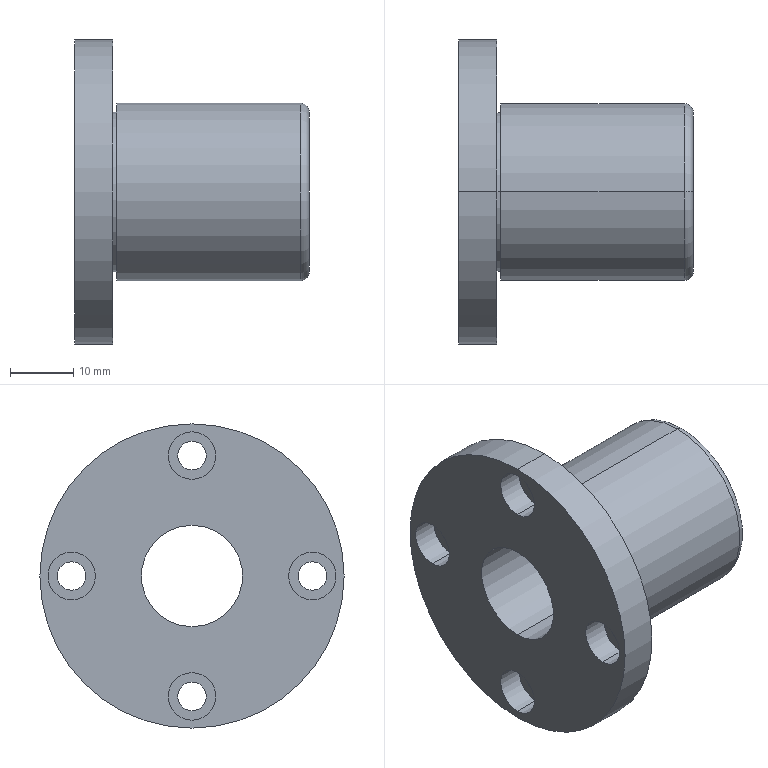Part | STEP file | MFMS16 | 1 solid | 34 faces | box 37 x 48 x 48 mm | volume 21555 mm3 | cylinder 24 | plane 8 | torus 2 | commonest cylinder face diameters 4.5 x8 7.5 x8 16 x2 25.2 x2 28 x2 48 x2
STEP:
#1=CARTESIAN_POINT('',(6.,0.,16.75));
#2=VERTEX_POINT('',#1);
#3=CARTESIAN_POINT('',(6.,0.,21.25));
#4=VERTEX_POINT('',#3);
#5=CARTESIAN_POINT('',(6.,0.,19.));
#6=DIRECTION('',(-1.,0.,0.));
#7=DIRECTION('',(0.,0.,1.));
#8=AXIS2_PLACEMENT_3D('',#5,#6,#7);
#9=CIRCLE('',#8,2.25);
#10=EDGE_CURVE('',#2,#4,#9,.T.);
#11=ORIENTED_EDGE('',*,*,#10,.F.);
#12=CARTESIAN_POINT('',(4.1,0.,16.75));
#13=VERTEX_POINT('',#12);
#14=CARTESIAN_POINT('',(6.,0.,16.75));
#15=DIRECTION('',(-1.,0.,0.));
#16=VECTOR('',#15,1000.);
#17=LINE('',#14,#16);
#18=EDGE_CURVE('',#2,#13,#17,.T.);
#19=ORIENTED_EDGE('',*,*,#18,.T.);
#20=CARTESIAN_POINT('',(4.1,0.,21.25));
#21=VERTEX_POINT('',#20);
#22=CARTESIAN_POINT('',(4.1,0.,19.));
#23=DIRECTION('',(-1.,0.,0.));
#24=DIRECTION('',(0.,0.,1.));
#25=AXIS2_PLACEMENT_3D('',#22,#23,#24);
#26=CIRCLE('',#25,2.25);
#27=EDGE_CURVE('',#13,#21,#26,.T.);
#28=ORIENTED_EDGE('',*,*,#27,.T.);
#29=CARTESIAN_POINT('',(6.,0.,21.25));
#30=DIRECTION('',(-1.,0.,0.));
#31=VECTOR('',#30,1000.);
#32=LINE('',#29,#31);
#33=EDGE_CURVE('',#4,#21,#32,.T.);
#34=ORIENTED_EDGE('',*,*,#33,.F.);
#35=EDGE_LOOP('',(#11,#19,#28,#34));
#36=FACE_OUTER_BOUND('',#35,.T.);
#37=CARTESIAN_POINT('',(6.,0.,19.));
#38=DIRECTION('',(-1.,0.,0.));
#39=DIRECTION('',(0.,0.,1.));
#40=AXIS2_PLACEMENT_3D('',#37,#38,#39);
#41=CYLINDRICAL_SURFACE('',#40,2.25);
#42=ADVANCED_FACE('',(#36),#41,.F.);
#43=CARTESIAN_POINT('',(4.1,0.,15.25));
#44=VERTEX_POINT('',#43);
#45=CARTESIAN_POINT('',(4.1,0.,22.75));
#46=VERTEX_POINT('',#45);
#47=CARTESIAN_POINT('',(4.1,0.,19.));
#48=DIRECTION('',(-1.,0.,0.));
#49=DIRECTION('',(0.,0.,1.));
#50=AXIS2_PLACEMENT_3D('',#47,#48,#49);
#51=CIRCLE('',#50,3.75);
#52=EDGE_CURVE('',#44,#46,#51,.T.);
#53=ORIENTED_EDGE('',*,*,#52,.F.);
#54=CARTESIAN_POINT('',(0.,0.,15.25));
#55=VERTEX_POINT('',#54);
#56=CARTESIAN_POINT('',(6.,0.,15.25));
#57=DIRECTION('',(-1.,0.,0.));
#58=VECTOR('',#57,1000.);
#59=LINE('',#56,#58);
#60=EDGE_CURVE('',#44,#55,#59,.T.);
#61=ORIENTED_EDGE('',*,*,#60,.T.);
#62=CARTESIAN_POINT('',(0.,0.,22.75));
#63=VERTEX_POINT('',#62);
#64=CARTESIAN_POINT('',(0.,0.,19.));
#65=DIRECTION('',(-1.,0.,0.));
#66=DIRECTION('',(0.,0.,1.));
#67=AXIS2_PLACEMENT_3D('',#64,#65,#66);
#68=CIRCLE('',#67,3.75);
#69=EDGE_CURVE('',#55,#63,#68,.T.);
#70=ORIENTED_EDGE('',*,*,#69,.T.);
#71=CARTESIAN_POINT('',(6.,0.,22.75));
#72=DIRECTION('',(-1.,0.,0.));
#73=VECTOR('',#72,1000.);
#74=LINE('',#71,#73);
#75=EDGE_CURVE('',#46,#63,#74,.T.);
#76=ORIENTED_EDGE('',*,*,#75,.F.);
#77=EDGE_LOOP('',(#53,#61,#70,#76));
#78=FACE_OUTER_BOUND('',#77,.T.);
#79=CARTESIAN_POINT('',(6.,0.,19.));
#80=DIRECTION('',(-1.,0.,0.));
#81=DIRECTION('',(0.,0.,1.));
#82=AXIS2_PLACEMENT_3D('',#79,#80,#81);
#83=CYLINDRICAL_SURFACE('',#82,3.75);
#84=ADVANCED_FACE('',(#78),#83,.F.);
#85=CARTESIAN_POINT('',(6.,-19.,-2.25));
#86=VERTEX_POINT('',#85);
#87=CARTESIAN_POINT('',(6.,-19.,2.25));
#88=VERTEX_POINT('',#87);
#89=CARTESIAN_POINT('',(6.,-19.,0.));
#90=DIRECTION('',(-1.,0.,0.));
#91=DIRECTION('',(0.,0.,1.));
#92=AXIS2_PLACEMENT_3D('',#89,#90,#91);
#93=CIRCLE('',#92,2.25);
#94=EDGE_CURVE('',#86,#88,#93,.T.);
#95=ORIENTED_EDGE('',*,*,#94,.F.);
#96=CARTESIAN_POINT('',(4.1,-19.,-2.25));
#97=VERTEX_POINT('',#96);
#98=CARTESIAN_POINT('',(6.,-19.,-2.25));
#99=DIRECTION('',(-1.,0.,0.));
#100=VECTOR('',#99,1000.);
#101=LINE('',#98,#100);
#102=EDGE_CURVE('',#86,#97,#101,.T.);
#103=ORIENTED_EDGE('',*,*,#102,.T.);
#104=CARTESIAN_POINT('',(4.1,-19.,2.25));
#105=VERTEX_POINT('',#104);
#106=CARTESIAN_POINT('',(4.1,-19.,0.));
#107=DIRECTION('',(-1.,0.,0.));
#108=DIRECTION('',(0.,0.,1.));
#109=AXIS2_PLACEMENT_3D('',#106,#107,#108);
#110=CIRCLE('',#109,2.25);
#111=EDGE_CURVE('',#97,#105,#110,.T.);
#112=ORIENTED_EDGE('',*,*,#111,.T.);
#113=CARTESIAN_POINT('',(6.,-19.,2.25));
#114=DIRECTION('',(-1.,0.,0.));
#115=VECTOR('',#114,1000.);
#116=LINE('',#113,#115);
#117=EDGE_CURVE('',#88,#105,#116,.T.);
#118=ORIENTED_EDGE('',*,*,#117,.F.);
#119=EDGE_LOOP('',(#95,#103,#112,#118));
#120=FACE_OUTER_BOUND('',#119,.T.);
#121=CARTESIAN_POINT('',(6.,-19.,0.));
#122=DIRECTION('',(-1.,0.,0.));
#123=DIRECTION('',(0.,0.,1.));
#124=AXIS2_PLACEMENT_3D('',#121,#122,#123);
#125=CYLINDRICAL_SURFACE('',#124,2.25);
#126=ADVANCED_FACE('',(#120),#125,.F.);
#127=CARTESIAN_POINT('',(4.1,-19.,-3.75));
#128=VERTEX_POINT('',#127);
#129=CARTESIAN_POINT('',(4.1,-19.,3.75));
#130=VERTEX_POINT('',#129);
#131=CARTESIAN_POINT('',(4.1,-19.,0.));
#132=DIRECTION('',(-1.,0.,0.));
#133=DIRECTION('',(0.,0.,1.));
#134=AXIS2_PLACEMENT_3D('',#131,#132,#133);
#135=CIRCLE('',#134,3.75);
#136=EDGE_CURVE('',#128,#130,#135,.T.);
#137=ORIENTED_EDGE('',*,*,#136,.F.);
#138=CARTESIAN_POINT('',(0.,-19.,-3.75));
#139=VERTEX_POINT('',#138);
#140=CARTESIAN_POINT('',(6.,-19.,-3.75));
#141=DIRECTION('',(-1.,0.,0.));
#142=VECTOR('',#141,1000.);
#143=LINE('',#140,#142);
#144=EDGE_CURVE('',#128,#139,#143,.T.);
#145=ORIENTED_EDGE('',*,*,#144,.T.);
#146=CARTESIAN_POINT('',(0.,-19.,3.75));
#147=VERTEX_POINT('',#146);
#148=CARTESIAN_POINT('',(0.,-19.,0.));
#149=DIRECTION('',(-1.,0.,0.));
#150=DIRECTION('',(0.,0.,1.));
#151=AXIS2_PLACEMENT_3D('',#148,#149,#150);
#152=CIRCLE('',#151,3.75);
#153=EDGE_CURVE('',#139,#147,#152,.T.);
#154=ORIENTED_EDGE('',*,*,#153,.T.);
#155=CARTESIAN_POINT('',(6.,-19.,3.75));
#156=DIRECTION('',(-1.,0.,0.));
#157=VECTOR('',#156,1000.);
#158=LINE('',#155,#157);
#159=EDGE_CURVE('',#130,#147,#158,.T.);
#160=ORIENTED_EDGE('',*,*,#159,.F.);
#161=EDGE_LOOP('',(#137,#145,#154,#160));
#162=FACE_OUTER_BOUND('',#161,.T.);
#163=CARTESIAN_POINT('',(6.,-19.,0.));
#164=DIRECTION('',(-1.,0.,0.));
#165=DIRECTION('',(0.,0.,1.));
#166=AXIS2_PLACEMENT_3D('',#163,#164,#165);
#167=CYLINDRICAL_SURFACE('',#166,3.75);
#168=ADVANCED_FACE('',(#162),#167,.F.);
#169=CARTESIAN_POINT('',(6.,0.,-21.25));
#170=VERTEX_POINT('',#169);
#171=CARTESIAN_POINT('',(6.,0.,-16.75));
#172=VERTEX_POINT('',#171);
#173=CARTESIAN_POINT('',(6.,0.,-19.));
#174=DIRECTION('',(-1.,0.,0.));
#175=DIRECTION('',(0.,0.,1.));
#176=AXIS2_PLACEMENT_3D('',#173,#174,#175);
#177=CIRCLE('',#176,2.25);
#178=EDGE_CURVE('',#170,#172,#177,.T.);
#179=ORIENTED_EDGE('',*,*,#178,.F.);
#180=CARTESIAN_POINT('',(4.1,0.,-21.25));
#181=VERTEX_POINT('',#180);
#182=CARTESIAN_POINT('',(6.,0.,-21.25));
#183=DIRECTION('',(-1.,0.,0.));
#184=VECTOR('',#183,1000.);
#185=LINE('',#182,#184);
#186=EDGE_CURVE('',#170,#181,#185,.T.);
#187=ORIENTED_EDGE('',*,*,#186,.T.);
#188=CARTESIAN_POINT('',(4.1,0.,-16.75));
#189=VERTEX_POINT('',#188);
#190=CARTESIAN_POINT('',(4.1,0.,-19.));
#191=DIRECTION('',(-1.,0.,0.));
#192=DIRECTION('',(0.,0.,1.));
#193=AXIS2_PLACEMENT_3D('',#190,#191,#192);
#194=CIRCLE('',#193,2.25);
#195=EDGE_CURVE('',#181,#189,#194,.T.);
#196=ORIENTED_EDGE('',*,*,#195,.T.);
#197=CARTESIAN_POINT('',(6.,0.,-16.75));
#198=DIRECTION('',(-1.,0.,0.));
#199=VECTOR('',#198,1000.);
#200=LINE('',#197,#199);
#201=EDGE_CURVE('',#172,#189,#200,.T.);
#202=ORIENTED_EDGE('',*,*,#201,.F.);
#203=EDGE_LOOP('',(#179,#187,#196,#202));
#204=FACE_OUTER_BOUND('',#203,.T.);
#205=CARTESIAN_POINT('',(6.,0.,-19.));
#206=DIRECTION('',(-1.,0.,0.));
#207=DIRECTION('',(0.,0.,1.));
#208=AXIS2_PLACEMENT_3D('',#205,#206,#207);
#209=CYLINDRICAL_SURFACE('',#208,2.25);
#210=ADVANCED_FACE('',(#204),#209,.F.);
#211=CARTESIAN_POINT('',(4.1,0.,-22.75));
#212=VERTEX_POINT('',#211);
#213=CARTESIAN_POINT('',(4.1,0.,-15.25));
#214=VERTEX_POINT('',#213);
#215=CARTESIAN_POINT('',(4.1,0.,-19.));
#216=DIRECTION('',(-1.,0.,0.));
#217=DIRECTION('',(0.,0.,1.));
#218=AXIS2_PLACEMENT_3D('',#215,#216,#217);
#219=CIRCLE('',#218,3.75);
#220=EDGE_CURVE('',#212,#214,#219,.T.);
#221=ORIENTED_EDGE('',*,*,#220,.F.);
#222=CARTESIAN_POINT('',(0.,0.,-22.75));
#223=VERTEX_POINT('',#222);
#224=CARTESIAN_POINT('',(6.,0.,-22.75));
#225=DIRECTION('',(-1.,0.,0.));
#226=VECTOR('',#225,1000.);
#227=LINE('',#224,#226);
#228=EDGE_CURVE('',#212,#223,#227,.T.);
#229=ORIENTED_EDGE('',*,*,#228,.T.);
#230=CARTESIAN_POINT('',(0.,0.,-15.25));
#231=VERTEX_POINT('',#230);
#232=CARTESIAN_POINT('',(0.,0.,-19.));
#233=DIRECTION('',(-1.,0.,0.));
#234=DIRECTION('',(0.,0.,1.));
#235=AXIS2_PLACEMENT_3D('',#232,#233,#234);
#236=CIRCLE('',#235,3.75);
#237=EDGE_CURVE('',#223,#231,#236,.T.);
#238=ORIENTED_EDGE('',*,*,#237,.T.);
#239=CARTESIAN_POINT('',(6.,0.,-15.25));
#240=DIRECTION('',(-1.,0.,0.));
#241=VECTOR('',#240,1000.);
#242=LINE('',#239,#241);
#243=EDGE_CURVE('',#214,#231,#242,.T.);
#244=ORIENTED_EDGE('',*,*,#243,.F.);
#245=EDGE_LOOP('',(#221,#229,#238,#244));
#246=FACE_OUTER_BOUND('',#245,.T.);
#247=CARTESIAN_POINT('',(6.,0.,-19.));
#248=DIRECTION('',(-1.,0.,0.));
#249=DIRECTION('',(0.,0.,1.));
#250=AXIS2_PLACEMENT_3D('',#247,#248,#249);
#251=CYLINDRICAL_SURFACE('',#250,3.75);
#252=ADVANCED_FACE('',(#246),#251,.F.);
#253=CARTESIAN_POINT('',(6.,19.,-2.25));
#254=VERTEX_POINT('',#253);
#255=CARTESIAN_POINT('',(6.,19.,2.25));
#256=VERTEX_POINT('',#255);
#257=CARTESIAN_POINT('',(6.,19.,0.));
#258=DIRECTION('',(-1.,0.,0.));
#259=DIRECTION('',(0.,0.,1.));
#260=AXIS2_PLACEMENT_3D('',#257,#258,#259);
#261=CIRCLE('',#260,2.25);
#262=EDGE_CURVE('',#254,#256,#261,.T.);
#263=ORIENTED_EDGE('',*,*,#262,.F.);
#264=CARTESIAN_POINT('',(4.1,19.,-2.25));
#265=VERTEX_POINT('',#264);
#266=CARTESIAN_POINT('',(6.,19.,-2.25));
#267=DIRECTION('',(-1.,0.,0.));
#268=VECTOR('',#267,1000.);
#269=LINE('',#266,#268);
#270=EDGE_CURVE('',#254,#265,#269,.T.);
#271=ORIENTED_EDGE('',*,*,#270,.T.);
#272=CARTESIAN_POINT('',(4.1,19.,2.25));
#273=VERTEX_POINT('',#272);
#274=CARTESIAN_POINT('',(4.1,19.,0.));
#275=DIRECTION('',(-1.,0.,0.));
#276=DIRECTION('',(0.,0.,1.));
#277=AXIS2_PLACEMENT_3D('',#274,#275,#276);
#278=CIRCLE('',#277,2.25);
#279=EDGE_CURVE('',#265,#273,#278,.T.);
#280=ORIENTED_EDGE('',*,*,#279,.T.);
#281=CARTESIAN_POINT('',(6.,19.,2.25));
#282=DIRECTION('',(-1.,0.,0.));
#283=VECTOR('',#282,1000.);
#284=LINE('',#281,#283);
#285=EDGE_CURVE('',#256,#273,#284,.T.);
#286=ORIENTED_EDGE('',*,*,#285,.F.);
#287=EDGE_LOOP('',(#263,#271,#280,#286));
#288=FACE_OUTER_BOUND('',#287,.T.);
#289=CARTESIAN_POINT('',(6.,19.,0.));
#290=DIRECTION('',(-1.,0.,0.));
#291=DIRECTION('',(0.,0.,1.));
#292=AXIS2_PLACEMENT_3D('',#289,#290,#291);
#293=CYLINDRICAL_SURFACE('',#292,2.25);
#294=ADVANCED_FACE('',(#288),#293,.F.);
#295=CARTESIAN_POINT('',(4.1,19.,-3.75));
#296=VERTEX_POINT('',#295);
#297=CARTESIAN_POINT('',(4.1,19.,3.75));
#298=VERTEX_POINT('',#297);
#299=CARTESIAN_POINT('',(4.1,19.,0.));
#300=DIRECTION('',(-1.,0.,0.));
#301=DIRECTION('',(0.,0.,1.));
#302=AXIS2_PLACEMENT_3D('',#299,#300,#301);
#303=CIRCLE('',#302,3.75);
#304=EDGE_CURVE('',#296,#298,#303,.T.);
#305=ORIENTED_EDGE('',*,*,#304,.F.);
#306=CARTESIAN_POINT('',(0.,19.,-3.75));
#307=VERTEX_POINT('',#306);
#308=CARTESIAN_POINT('',(6.,19.,-3.75));
#309=DIRECTION('',(-1.,0.,0.));
#310=VECTOR('',#309,1000.);
#311=LINE('',#308,#310);
#312=EDGE_CURVE('',#296,#307,#311,.T.);
#313=ORIENTED_EDGE('',*,*,#312,.T.);
#314=CARTESIAN_POINT('',(0.,19.,3.75));
#315=VERTEX_POINT('',#314);
#316=CARTESIAN_POINT('',(0.,19.,0.));
#317=DIRECTION('',(-1.,0.,0.));
#318=DIRECTION('',(0.,0.,1.));
#319=AXIS2_PLACEMENT_3D('',#316,#317,#318);
#320=CIRCLE('',#319,3.75);
#321=EDGE_CURVE('',#307,#315,#320,.T.);
#322=ORIENTED_EDGE('',*,*,#321,.T.);
#323=CARTESIAN_POINT('',(6.,19.,3.75));
#324=DIRECTION('',(-1.,0.,0.));
#325=VECTOR('',#324,1000.);
#326=LINE('',#323,#325);
#327=EDGE_CURVE('',#298,#315,#326,.T.);
#328=ORIENTED_EDGE('',*,*,#327,.F.);
#329=EDGE_LOOP('',(#305,#313,#322,#328));
#330=FACE_OUTER_BOUND('',#329,.T.);
#331=CARTESIAN_POINT('',(6.,19.,0.));
#332=DIRECTION('',(-1.,0.,0.));
#333=DIRECTION('',(0.,0.,1.));
#334=AXIS2_PLACEMENT_3D('',#331,#332,#333);
#335=CYLINDRICAL_SURFACE('',#334,3.75);
#336=ADVANCED_FACE('',(#330),#335,.F.);
#337=CARTESIAN_POINT('',(6.6,0.,12.6));
#338=VERTEX_POINT('',#337);
#339=CARTESIAN_POINT('',(6.6,0.,-12.6));
#340=VERTEX_POINT('',#339);
#341=CARTESIAN_POINT('',(6.6,0.,0.));
#342=DIRECTION('',(-1.,0.,0.));
#343=DIRECTION('',(0.,0.,1.));
#344=AXIS2_PLACEMENT_3D('',#341,#342,#343);
#345=CIRCLE('',#344,12.6);
#346=EDGE_CURVE('',#338,#340,#345,.T.);
#347=ORIENTED_EDGE('',*,*,#346,.T.);
#348=CARTESIAN_POINT('',(6.,0.,-12.6));
#349=VERTEX_POINT('',#348);
#350=CARTESIAN_POINT('',(37.,0.,-12.6));
#351=DIRECTION('',(-1.,0.,0.));
#352=VECTOR('',#351,1000.);
#353=LINE('',#350,#352);
#354=EDGE_CURVE('',#340,#349,#353,.T.);
#355=ORIENTED_EDGE('',*,*,#354,.T.);
#356=CARTESIAN_POINT('',(6.,0.,12.6));
#357=VERTEX_POINT('',#356);
#358=CARTESIAN_POINT('',(6.,0.,0.));
#359=DIRECTION('',(-1.,0.,0.));
#360=DIRECTION('',(0.,0.,1.));
#361=AXIS2_PLACEMENT_3D('',#358,#359,#360);
#362=CIRCLE('',#361,12.6);
#363=EDGE_CURVE('',#357,#349,#362,.T.);
#364=ORIENTED_EDGE('',*,*,#363,.F.);
#365=CARTESIAN_POINT('',(37.,0.,12.6));
#366=DIRECTION('',(-1.,0.,0.));
#367=VECTOR('',#366,1000.);
#368=LINE('',#365,#367);
#369=EDGE_CURVE('',#338,#357,#368,.T.);
#370=ORIENTED_EDGE('',*,*,#369,.F.);
#371=EDGE_LOOP('',(#347,#355,#364,#370));
#372=FACE_OUTER_BOUND('',#371,.T.);
#373=CARTESIAN_POINT('',(37.,0.,0.));
#374=DIRECTION('',(-1.,0.,0.));
#375=DIRECTION('',(0.,0.,1.));
#376=AXIS2_PLACEMENT_3D('',#373,#374,#375);
#377=CYLINDRICAL_SURFACE('',#376,12.6);
#378=ADVANCED_FACE('',(#372),#377,.T.);
#379=CARTESIAN_POINT('',(35.6,0.,14.));
#380=VERTEX_POINT('',#379);
#381=CARTESIAN_POINT('',(35.6,0.,-14.));
#382=VERTEX_POINT('',#381);
#383=CARTESIAN_POINT('',(35.6,0.,0.));
#384=DIRECTION('',(-1.,0.,0.));
#385=DIRECTION('',(0.,0.,1.));
#386=AXIS2_PLACEMENT_3D('',#383,#384,#385);
#387=CIRCLE('',#386,14.);
#388=EDGE_CURVE('',#380,#382,#387,.T.);
#389=ORIENTED_EDGE('',*,*,#388,.T.);
#390=CARTESIAN_POINT('',(6.6,0.,-14.));
#391=VERTEX_POINT('',#390);
#392=CARTESIAN_POINT('',(37.,0.,-14.));
#393=DIRECTION('',(-1.,0.,0.));
#394=VECTOR('',#393,1000.);
#395=LINE('',#392,#394);
#396=EDGE_CURVE('',#382,#391,#395,.T.);
#397=ORIENTED_EDGE('',*,*,#396,.T.);
#398=CARTESIAN_POINT('',(6.6,0.,14.));
#399=VERTEX_POINT('',#398);
#400=CARTESIAN_POINT('',(6.6,0.,0.));
#401=DIRECTION('',(-1.,0.,0.));
#402=DIRECTION('',(0.,0.,1.));
#403=AXIS2_PLACEMENT_3D('',#400,#401,#402);
#404=CIRCLE('',#403,14.);
#405=EDGE_CURVE('',#399,#391,#404,.T.);
#406=ORIENTED_EDGE('',*,*,#405,.F.);
#407=CARTESIAN_POINT('',(37.,0.,14.));
#408=DIRECTION('',(-1.,0.,0.));
#409=VECTOR('',#408,1000.);
#410=LINE('',#407,#409);
#411=EDGE_CURVE('',#380,#399,#410,.T.);
#412=ORIENTED_EDGE('',*,*,#411,.F.);
#413=EDGE_LOOP('',(#389,#397,#406,#412));
#414=FACE_OUTER_BOUND('',#413,.T.);
#415=CARTESIAN_POINT('',(37.,0.,0.));
#416=DIRECTION('',(-1.,0.,0.));
#417=DIRECTION('',(0.,0.,1.));
#418=AXIS2_PLACEMENT_3D('',#415,#416,#417);
#419=CYLINDRICAL_SURFACE('',#418,14.);
#420=ADVANCED_FACE('',(#414),#419,.T.);
#421=CARTESIAN_POINT('',(37.,0.,12.6));
#422=VERTEX_POINT('',#421);
#423=CARTESIAN_POINT('',(37.,0.,-12.6));
#424=VERTEX_POINT('',#423);
#425=CARTESIAN_POINT('',(37.,0.,0.));
#426=DIRECTION('',(-1.,0.,0.));
#427=DIRECTION('',(0.,0.,1.));
#428=AXIS2_PLACEMENT_3D('',#425,#426,#427);
#429=CIRCLE('',#428,12.6);
#430=EDGE_CURVE('',#422,#424,#429,.T.);
#431=ORIENTED_EDGE('',*,*,#430,.T.);
#432=CARTESIAN_POINT('',(35.6,0.,-12.6));
#433=DIRECTION('',(0.,1.,0.));
#434=DIRECTION('',(0.,0.,1.));
#435=AXIS2_PLACEMENT_3D('',#432,#433,#434);
#436=CIRCLE('',#435,1.4);
#437=EDGE_CURVE('',#424,#382,#436,.T.);
#438=ORIENTED_EDGE('',*,*,#437,.T.);
#439=ORIENTED_EDGE('',*,*,#388,.F.);
#440=CARTESIAN_POINT('',(35.6,0.,12.6));
#441=DIRECTION('',(0.,-1.,0.));
#442=DIRECTION('',(0.,0.,-1.));
#443=AXIS2_PLACEMENT_3D('',#440,#441,#442);
#444=CIRCLE('',#443,1.4);
#445=EDGE_CURVE('',#422,#380,#444,.T.);
#446=ORIENTED_EDGE('',*,*,#445,.F.);
#447=EDGE_LOOP('',(#431,#438,#439,#446));
#448=FACE_OUTER_BOUND('',#447,.T.);
#449=CARTESIAN_POINT('',(35.6,0.,0.));
#450=DIRECTION('',(-1.,0.,0.));
#451=DIRECTION('',(0.,0.,1.));
#452=AXIS2_PLACEMENT_3D('',#449,#450,#451);
#453=TOROIDAL_SURFACE('',#452,12.6,1.4);
#454=ADVANCED_FACE('',(#448),#453,.T.);
#455=CARTESIAN_POINT('',(37.,0.,-8.));
#456=VERTEX_POINT('',#455);
#457=CARTESIAN_POINT('',(37.,0.,8.));
#458=VERTEX_POINT('',#457);
#459=CARTESIAN_POINT('',(37.,0.,0.));
#460=DIRECTION('',(-1.,0.,0.));
#461=DIRECTION('',(0.,0.,1.));
#462=AXIS2_PLACEMENT_3D('',#459,#460,#461);
#463=CIRCLE('',#462,8.);
#464=EDGE_CURVE('',#456,#458,#463,.T.);
#465=ORIENTED_EDGE('',*,*,#464,.F.);
#466=CARTESIAN_POINT('',(0.,0.,-8.));
#467=VERTEX_POINT('',#466);
#468=CARTESIAN_POINT('',(37.,0.,-8.));
#469=DIRECTION('',(-1.,0.,0.));
#470=VECTOR('',#469,1000.);
#471=LINE('',#468,#470);
#472=EDGE_CURVE('',#456,#467,#471,.T.);
#473=ORIENTED_EDGE('',*,*,#472,.T.);
#474=CARTESIAN_POINT('',(0.,0.,8.));
#475=VERTEX_POINT('',#474);
#476=CARTESIAN_POINT('',(0.,0.,0.));
#477=DIRECTION('',(-1.,0.,0.));
#478=DIRECTION('',(0.,0.,1.));
#479=AXIS2_PLACEMENT_3D('',#476,#477,#478);
#480=CIRCLE('',#479,8.);
#481=EDGE_CURVE('',#467,#475,#480,.T.);
#482=ORIENTED_EDGE('',*,*,#481,.T.);
#483=CARTESIAN_POINT('',(37.,0.,8.));
#484=DIRECTION('',(-1.,0.,0.));
#485=VECTOR('',#484,1000.);
#486=LINE('',#483,#485);
#487=EDGE_CURVE('',#458,#475,#486,.T.);
#488=ORIENTED_EDGE('',*,*,#487,.F.);
#489=EDGE_LOOP('',(#465,#473,#482,#488));
#490=FACE_OUTER_BOUND('',#489,.T.);
#491=CARTESIAN_POINT('',(37.,0.,0.));
#492=DIRECTION('',(-1.,0.,0.));
#493=DIRECTION('',(0.,0.,1.));
#494=AXIS2_PLACEMENT_3D('',#491,#492,#493);
#495=CYLINDRICAL_SURFACE('',#494,8.);
#496=ADVANCED_FACE('',(#490),#495,.F.);
#497=CARTESIAN_POINT('',(6.,0.,24.));
#498=VERTEX_POINT('',#497);
#499=CARTESIAN_POINT('',(6.,0.,-24.));
#500=VERTEX_POINT('',#499);
#501=CARTESIAN_POINT('',(6.,0.,0.));
#502=DIRECTION('',(-1.,0.,0.));
#503=DIRECTION('',(0.,0.,1.));
#504=AXIS2_PLACEMENT_3D('',#501,#502,#503);
#505=CIRCLE('',#504,24.);
#506=EDGE_CURVE('',#498,#500,#505,.T.);
#507=ORIENTED_EDGE('',*,*,#506,.T.);
#508=CARTESIAN_POINT('',(0.,0.,-24.));
#509=VERTEX_POINT('',#508);
#510=CARTESIAN_POINT('',(37.,0.,-24.));
#511=DIRECTION('',(-1.,0.,0.));
#512=VECTOR('',#511,1000.);
#513=LINE('',#510,#512);
#514=EDGE_CURVE('',#500,#509,#513,.T.);
#515=ORIENTED_EDGE('',*,*,#514,.T.);
#516=CARTESIAN_POINT('',(0.,0.,24.));
#517=VERTEX_POINT('',#516);
#518=CARTESIAN_POINT('',(0.,0.,0.));
#519=DIRECTION('',(-1.,0.,0.));
#520=DIRECTION('',(0.,0.,1.));
#521=AXIS2_PLACEMENT_3D('',#518,#519,#520);
#522=CIRCLE('',#521,24.);
#523=EDGE_CURVE('',#517,#509,#522,.T.);
#524=ORIENTED_EDGE('',*,*,#523,.F.);
#525=CARTESIAN_POINT('',(37.,0.,24.));
#526=DIRECTION('',(-1.,0.,0.));
#527=VECTOR('',#526,1000.);
#528=LINE('',#525,#527);
#529=EDGE_CURVE('',#498,#517,#528,.T.);
#530=ORIENTED_EDGE('',*,*,#529,.F.);
#531=EDGE_LOOP('',(#507,#515,#524,#530));
#532=FACE_OUTER_BOUND('',#531,.T.);
#533=CARTESIAN_POINT('',(37.,0.,0.));
#534=DIRECTION('',(-1.,0.,0.));
#535=DIRECTION('',(0.,0.,1.));
#536=AXIS2_PLACEMENT_3D('',#533,#534,#535);
#537=CYLINDRICAL_SURFACE('',#536,24.);
#538=ADVANCED_FACE('',(#532),#537,.T.);
#539=CARTESIAN_POINT('',(0.,-19.,0.));
#540=DIRECTION('',(-1.,0.,0.));
#541=DIRECTION('',(0.,0.,1.));
#542=AXIS2_PLACEMENT_3D('',#539,#540,#541);
#543=CIRCLE('',#542,3.75);
#544=EDGE_CURVE('',#147,#139,#543,.T.);
#545=ORIENTED_EDGE('',*,*,#544,.F.);
#546=ORIENTED_EDGE('',*,*,#153,.F.);
#547=EDGE_LOOP('',(#545,#546));
#548=FACE_BOUND('',#547,.T.);
#549=CARTESIAN_POINT('',(0.,19.,0.));
#550=DIRECTION('',(-1.,0.,0.));
#551=DIRECTION('',(0.,0.,1.));
#552=AXIS2_PLACEMENT_3D('',#549,#550,#551);
#553=CIRCLE('',#552,3.75);
#554=EDGE_CURVE('',#315,#307,#553,.T.);
#555=ORIENTED_EDGE('',*,*,#554,.F.);
#556=ORIENTED_EDGE('',*,*,#321,.F.);
#557=EDGE_LOOP('',(#555,#556));
#558=FACE_BOUND('',#557,.T.);
#559=CARTESIAN_POINT('',(0.,0.,0.));
#560=DIRECTION('',(-1.,0.,0.));
#561=DIRECTION('',(0.,0.,1.));
#562=AXIS2_PLACEMENT_3D('',#559,#560,#561);
#563=CIRCLE('',#562,8.);
#564=EDGE_CURVE('',#475,#467,#563,.T.);
#565=ORIENTED_EDGE('',*,*,#564,.F.);
#566=ORIENTED_EDGE('',*,*,#481,.F.);
#567=EDGE_LOOP('',(#565,#566));
#568=FACE_BOUND('',#567,.T.);
#569=ORIENTED_EDGE('',*,*,#523,.T.);
#570=CARTESIAN_POINT('',(0.,0.,0.));
#571=DIRECTION('',(-1.,0.,0.));
#572=DIRECTION('',(0.,0.,1.));
#573=AXIS2_PLACEMENT_3D('',#570,#571,#572);
#574=CIRCLE('',#573,24.);
#575=EDGE_CURVE('',#509,#517,#574,.T.);
#576=ORIENTED_EDGE('',*,*,#575,.T.);
#577=EDGE_LOOP('',(#569,#576));
#578=FACE_OUTER_BOUND('',#577,.T.);
#579=CARTESIAN_POINT('',(0.,0.,-19.));
#580=DIRECTION('',(-1.,0.,0.));
#581=DIRECTION('',(0.,0.,1.));
#582=AXIS2_PLACEMENT_3D('',#579,#580,#581);
#583=CIRCLE('',#582,3.75);
#584=EDGE_CURVE('',#231,#223,#583,.T.);
#585=ORIENTED_EDGE('',*,*,#584,.F.);
#586=ORIENTED_EDGE('',*,*,#237,.F.);
#587=EDGE_LOOP('',(#585,#586));
#588=FACE_BOUND('',#587,.T.);
#589=CARTESIAN_POINT('',(0.,0.,19.));
#590=DIRECTION('',(-1.,0.,0.));
#591=DIRECTION('',(0.,0.,1.));
#592=AXIS2_PLACEMENT_3D('',#589,#590,#591);
#593=CIRCLE('',#592,3.75);
#594=EDGE_CURVE('',#63,#55,#593,.T.);
#595=ORIENTED_EDGE('',*,*,#594,.F.);
#596=ORIENTED_EDGE('',*,*,#69,.F.);
#597=EDGE_LOOP('',(#595,#596));
#598=FACE_BOUND('',#597,.T.);
#599=CARTESIAN_POINT('',(0.,24.,0.));
#600=DIRECTION('',(1.,0.,0.));
#601=DIRECTION('',(0.,0.,-1.));
#602=AXIS2_PLACEMENT_3D('',#599,#600,#601);
#603=PLANE('',#602);
#604=ADVANCED_FACE('',(#548,#558,#568,#578,#588,#598),#603,.F.);
#605=CARTESIAN_POINT('',(6.,-19.,0.));
#606=DIRECTION('',(-1.,0.,0.));
#607=DIRECTION('',(0.,0.,1.));
#608=AXIS2_PLACEMENT_3D('',#605,#606,#607);
#609=CIRCLE('',#608,2.25);
#610=EDGE_CURVE('',#88,#86,#609,.T.);
#611=ORIENTED_EDGE('',*,*,#610,.T.);
#612=ORIENTED_EDGE('',*,*,#94,.T.);
#613=EDGE_LOOP('',(#611,#612));
#614=FACE_BOUND('',#613,.T.);
#615=CARTESIAN_POINT('',(6.,19.,0.));
#616=DIRECTION('',(-1.,0.,0.));
#617=DIRECTION('',(0.,0.,1.));
#618=AXIS2_PLACEMENT_3D('',#615,#616,#617);
#619=CIRCLE('',#618,2.25);
#620=EDGE_CURVE('',#256,#254,#619,.T.);
#621=ORIENTED_EDGE('',*,*,#620,.T.);
#622=ORIENTED_EDGE('',*,*,#262,.T.);
#623=EDGE_LOOP('',(#621,#622));
#624=FACE_BOUND('',#623,.T.);
#625=ORIENTED_EDGE('',*,*,#506,.F.);
#626=CARTESIAN_POINT('',(6.,0.,0.));
#627=DIRECTION('',(-1.,0.,0.));
#628=DIRECTION('',(0.,0.,1.));
#629=AXIS2_PLACEMENT_3D('',#626,#627,#628);
#630=CIRCLE('',#629,24.);
#631=EDGE_CURVE('',#500,#498,#630,.T.);
#632=ORIENTED_EDGE('',*,*,#631,.F.);
#633=EDGE_LOOP('',(#625,#632));
#634=FACE_OUTER_BOUND('',#633,.T.);
#635=ORIENTED_EDGE('',*,*,#363,.T.);
#636=CARTESIAN_POINT('',(6.,0.,0.));
#637=DIRECTION('',(-1.,0.,0.));
#638=DIRECTION('',(0.,0.,1.));
#639=AXIS2_PLACEMENT_3D('',#636,#637,#638);
#640=CIRCLE('',#639,12.6);
#641=EDGE_CURVE('',#349,#357,#640,.T.);
#642=ORIENTED_EDGE('',*,*,#641,.T.);
#643=EDGE_LOOP('',(#635,#642));
#644=FACE_BOUND('',#643,.T.);
#645=CARTESIAN_POINT('',(6.,0.,-19.));
#646=DIRECTION('',(-1.,0.,0.));
#647=DIRECTION('',(0.,0.,1.));
#648=AXIS2_PLACEMENT_3D('',#645,#646,#647);
#649=CIRCLE('',#648,2.25);
#650=EDGE_CURVE('',#172,#170,#649,.T.);
#651=ORIENTED_EDGE('',*,*,#650,.T.);
#652=ORIENTED_EDGE('',*,*,#178,.T.);
#653=EDGE_LOOP('',(#651,#652));
#654=FACE_BOUND('',#653,.T.);
#655=CARTESIAN_POINT('',(6.,0.,19.));
#656=DIRECTION('',(-1.,0.,0.));
#657=DIRECTION('',(0.,0.,1.));
#658=AXIS2_PLACEMENT_3D('',#655,#656,#657);
#659=CIRCLE('',#658,2.25);
#660=EDGE_CURVE('',#4,#2,#659,.T.);
#661=ORIENTED_EDGE('',*,*,#660,.T.);
#662=ORIENTED_EDGE('',*,*,#10,.T.);
#663=EDGE_LOOP('',(#661,#662));
#664=FACE_BOUND('',#663,.T.);
#665=CARTESIAN_POINT('',(6.,12.6,0.));
#666=DIRECTION('',(-1.,0.,0.));
#667=DIRECTION('',(0.,0.,1.));
#668=AXIS2_PLACEMENT_3D('',#665,#666,#667);
#669=PLANE('',#668);
#670=ADVANCED_FACE('',(#614,#624,#634,#644,#654,#664),#669,.F.);
#671=ORIENTED_EDGE('',*,*,#514,.F.);
#672=ORIENTED_EDGE('',*,*,#631,.T.);
#673=ORIENTED_EDGE('',*,*,#529,.T.);
#674=ORIENTED_EDGE('',*,*,#575,.F.);
#675=EDGE_LOOP('',(#671,#672,#673,#674));
#676=FACE_OUTER_BOUND('',#675,.T.);
#677=CARTESIAN_POINT('',(37.,0.,0.));
#678=DIRECTION('',(-1.,0.,0.));
#679=DIRECTION('',(0.,0.,1.));
#680=AXIS2_PLACEMENT_3D('',#677,#678,#679);
#681=CYLINDRICAL_SURFACE('',#680,24.);
#682=ADVANCED_FACE('',(#676),#681,.T.);
#683=ORIENTED_EDGE('',*,*,#472,.F.);
#684=CARTESIAN_POINT('',(37.,0.,0.));
#685=DIRECTION('',(-1.,0.,0.));
#686=DIRECTION('',(0.,0.,1.));
#687=AXIS2_PLACEMENT_3D('',#684,#685,#686);
#688=CIRCLE('',#687,8.);
#689=EDGE_CURVE('',#458,#456,#688,.T.);
#690=ORIENTED_EDGE('',*,*,#689,.F.);
#691=ORIENTED_EDGE('',*,*,#487,.T.);
#692=ORIENTED_EDGE('',*,*,#564,.T.);
#693=EDGE_LOOP('',(#683,#690,#691,#692));
#694=FACE_OUTER_BOUND('',#693,.T.);
#695=CARTESIAN_POINT('',(37.,0.,0.));
#696=DIRECTION('',(-1.,0.,0.));
#697=DIRECTION('',(0.,0.,1.));
#698=AXIS2_PLACEMENT_3D('',#695,#696,#697);
#699=CYLINDRICAL_SURFACE('',#698,8.);
#700=ADVANCED_FACE('',(#694),#699,.F.);
#701=ORIENTED_EDGE('',*,*,#430,.F.);
#702=CARTESIAN_POINT('',(37.,0.,0.));
#703=DIRECTION('',(-1.,0.,0.));
#704=DIRECTION('',(0.,0.,1.));
#705=AXIS2_PLACEMENT_3D('',#702,#703,#704);
#706=CIRCLE('',#705,12.6);
#707=EDGE_CURVE('',#424,#422,#706,.T.);
#708=ORIENTED_EDGE('',*,*,#707,.F.);
#709=EDGE_LOOP('',(#701,#708));
#710=FACE_OUTER_BOUND('',#709,.T.);
#711=ORIENTED_EDGE('',*,*,#689,.T.);
#712=ORIENTED_EDGE('',*,*,#464,.T.);
#713=EDGE_LOOP('',(#711,#712));
#714=FACE_BOUND('',#713,.T.);
#715=CARTESIAN_POINT('',(37.,8.,0.));
#716=DIRECTION('',(-1.,0.,0.));
#717=DIRECTION('',(0.,0.,1.));
#718=AXIS2_PLACEMENT_3D('',#715,#716,#717);
#719=PLANE('',#718);
#720=ADVANCED_FACE('',(#710,#714),#719,.F.);
#721=ORIENTED_EDGE('',*,*,#437,.F.);
#722=ORIENTED_EDGE('',*,*,#707,.T.);
#723=ORIENTED_EDGE('',*,*,#445,.T.);
#724=CARTESIAN_POINT('',(35.6,0.,0.));
#725=DIRECTION('',(-1.,0.,0.));
#726=DIRECTION('',(0.,0.,1.));
#727=AXIS2_PLACEMENT_3D('',#724,#725,#726);
#728=CIRCLE('',#727,14.);
#729=EDGE_CURVE('',#382,#380,#728,.T.);
#730=ORIENTED_EDGE('',*,*,#729,.F.);
#731=EDGE_LOOP('',(#721,#722,#723,#730));
#732=FACE_OUTER_BOUND('',#731,.T.);
#733=CARTESIAN_POINT('',(35.6,0.,0.));
#734=DIRECTION('',(-1.,0.,0.));
#735=DIRECTION('',(0.,0.,1.));
#736=AXIS2_PLACEMENT_3D('',#733,#734,#735);
#737=TOROIDAL_SURFACE('',#736,12.6,1.4);
#738=ADVANCED_FACE('',(#732),#737,.T.);
#739=ORIENTED_EDGE('',*,*,#396,.F.);
#740=ORIENTED_EDGE('',*,*,#729,.T.);
#741=ORIENTED_EDGE('',*,*,#411,.T.);
#742=CARTESIAN_POINT('',(6.6,0.,0.));
#743=DIRECTION('',(-1.,0.,0.));
#744=DIRECTION('',(0.,0.,1.));
#745=AXIS2_PLACEMENT_3D('',#742,#743,#744);
#746=CIRCLE('',#745,14.);
#747=EDGE_CURVE('',#391,#399,#746,.T.);
#748=ORIENTED_EDGE('',*,*,#747,.F.);
#749=EDGE_LOOP('',(#739,#740,#741,#748));
#750=FACE_OUTER_BOUND('',#749,.T.);
#751=CARTESIAN_POINT('',(37.,0.,0.));
#752=DIRECTION('',(-1.,0.,0.));
#753=DIRECTION('',(0.,0.,1.));
#754=AXIS2_PLACEMENT_3D('',#751,#752,#753);
#755=CYLINDRICAL_SURFACE('',#754,14.);
#756=ADVANCED_FACE('',(#750),#755,.T.);
#757=ORIENTED_EDGE('',*,*,#346,.F.);
#758=CARTESIAN_POINT('',(6.6,0.,0.));
#759=DIRECTION('',(-1.,0.,0.));
#760=DIRECTION('',(0.,0.,1.));
#761=AXIS2_PLACEMENT_3D('',#758,#759,#760);
#762=CIRCLE('',#761,12.6);
#763=EDGE_CURVE('',#340,#338,#762,.T.);
#764=ORIENTED_EDGE('',*,*,#763,.F.);
#765=EDGE_LOOP('',(#757,#764));
#766=FACE_BOUND('',#765,.T.);
#767=ORIENTED_EDGE('',*,*,#405,.T.);
#768=ORIENTED_EDGE('',*,*,#747,.T.);
#769=EDGE_LOOP('',(#767,#768));
#770=FACE_OUTER_BOUND('',#769,.T.);
#771=CARTESIAN_POINT('',(6.6,14.,0.));
#772=DIRECTION('',(1.,0.,0.));
#773=DIRECTION('',(0.,0.,-1.));
#774=AXIS2_PLACEMENT_3D('',#771,#772,#773);
#775=PLANE('',#774);
#776=ADVANCED_FACE('',(#766,#770),#775,.F.);
#777=ORIENTED_EDGE('',*,*,#354,.F.);
#778=ORIENTED_EDGE('',*,*,#763,.T.);
#779=ORIENTED_EDGE('',*,*,#369,.T.);
#780=ORIENTED_EDGE('',*,*,#641,.F.);
#781=EDGE_LOOP('',(#777,#778,#779,#780));
#782=FACE_OUTER_BOUND('',#781,.T.);
#783=CARTESIAN_POINT('',(37.,0.,0.));
#784=DIRECTION('',(-1.,0.,0.));
#785=DIRECTION('',(0.,0.,1.));
#786=AXIS2_PLACEMENT_3D('',#783,#784,#785);
#787=CYLINDRICAL_SURFACE('',#786,12.6);
#788=ADVANCED_FACE('',(#782),#787,.T.);
#789=ORIENTED_EDGE('',*,*,#312,.F.);
#790=CARTESIAN_POINT('',(4.1,19.,0.));
#791=DIRECTION('',(-1.,0.,0.));
#792=DIRECTION('',(0.,0.,1.));
#793=AXIS2_PLACEMENT_3D('',#790,#791,#792);
#794=CIRCLE('',#793,3.75);
#795=EDGE_CURVE('',#298,#296,#794,.T.);
#796=ORIENTED_EDGE('',*,*,#795,.F.);
#797=ORIENTED_EDGE('',*,*,#327,.T.);
#798=ORIENTED_EDGE('',*,*,#554,.T.);
#799=EDGE_LOOP('',(#789,#796,#797,#798));
#800=FACE_OUTER_BOUND('',#799,.T.);
#801=CARTESIAN_POINT('',(6.,19.,0.));
#802=DIRECTION('',(-1.,0.,0.));
#803=DIRECTION('',(0.,0.,1.));
#804=AXIS2_PLACEMENT_3D('',#801,#802,#803);
#805=CYLINDRICAL_SURFACE('',#804,3.75);
#806=ADVANCED_FACE('',(#800),#805,.F.);
#807=ORIENTED_EDGE('',*,*,#795,.T.);
#808=ORIENTED_EDGE('',*,*,#304,.T.);
#809=EDGE_LOOP('',(#807,#808));
#810=FACE_OUTER_BOUND('',#809,.T.);
#811=CARTESIAN_POINT('',(4.1,19.,0.));
#812=DIRECTION('',(-1.,0.,0.));
#813=DIRECTION('',(0.,0.,1.));
#814=AXIS2_PLACEMENT_3D('',#811,#812,#813);
#815=CIRCLE('',#814,2.25);
#816=EDGE_CURVE('',#273,#265,#815,.T.);
#817=ORIENTED_EDGE('',*,*,#816,.F.);
#818=ORIENTED_EDGE('',*,*,#279,.F.);
#819=EDGE_LOOP('',(#817,#818));
#820=FACE_BOUND('',#819,.T.);
#821=CARTESIAN_POINT('',(4.1,22.75,0.));
#822=DIRECTION('',(-1.,0.,0.));
#823=DIRECTION('',(0.,0.,1.));
#824=AXIS2_PLACEMENT_3D('',#821,#822,#823);
#825=PLANE('',#824);
#826=ADVANCED_FACE('',(#810,#820),#825,.T.);
#827=ORIENTED_EDGE('',*,*,#270,.F.);
#828=ORIENTED_EDGE('',*,*,#620,.F.);
#829=ORIENTED_EDGE('',*,*,#285,.T.);
#830=ORIENTED_EDGE('',*,*,#816,.T.);
#831=EDGE_LOOP('',(#827,#828,#829,#830));
#832=FACE_OUTER_BOUND('',#831,.T.);
#833=CARTESIAN_POINT('',(6.,19.,0.));
#834=DIRECTION('',(-1.,0.,0.));
#835=DIRECTION('',(0.,0.,1.));
#836=AXIS2_PLACEMENT_3D('',#833,#834,#835);
#837=CYLINDRICAL_SURFACE('',#836,2.25);
#838=ADVANCED_FACE('',(#832),#837,.F.);
#839=ORIENTED_EDGE('',*,*,#228,.F.);
#840=CARTESIAN_POINT('',(4.1,0.,-19.));
#841=DIRECTION('',(-1.,0.,0.));
#842=DIRECTION('',(0.,0.,1.));
#843=AXIS2_PLACEMENT_3D('',#840,#841,#842);
#844=CIRCLE('',#843,3.75);
#845=EDGE_CURVE('',#214,#212,#844,.T.);
#846=ORIENTED_EDGE('',*,*,#845,.F.);
#847=ORIENTED_EDGE('',*,*,#243,.T.);
#848=ORIENTED_EDGE('',*,*,#584,.T.);
#849=EDGE_LOOP('',(#839,#846,#847,#848));
#850=FACE_OUTER_BOUND('',#849,.T.);
#851=CARTESIAN_POINT('',(6.,0.,-19.));
#852=DIRECTION('',(-1.,0.,0.));
#853=DIRECTION('',(0.,0.,1.));
#854=AXIS2_PLACEMENT_3D('',#851,#852,#853);
#855=CYLINDRICAL_SURFACE('',#854,3.75);
#856=ADVANCED_FACE('',(#850),#855,.F.);
#857=ORIENTED_EDGE('',*,*,#845,.T.);
#858=ORIENTED_EDGE('',*,*,#220,.T.);
#859=EDGE_LOOP('',(#857,#858));
#860=FACE_OUTER_BOUND('',#859,.T.);
#861=CARTESIAN_POINT('',(4.1,0.,-19.));
#862=DIRECTION('',(-1.,0.,0.));
#863=DIRECTION('',(0.,0.,1.));
#864=AXIS2_PLACEMENT_3D('',#861,#862,#863);
#865=CIRCLE('',#864,2.25);
#866=EDGE_CURVE('',#189,#181,#865,.T.);
#867=ORIENTED_EDGE('',*,*,#866,.F.);
#868=ORIENTED_EDGE('',*,*,#195,.F.);
#869=EDGE_LOOP('',(#867,#868));
#870=FACE_BOUND('',#869,.T.);
#871=CARTESIAN_POINT('',(4.1,3.75,-19.));
#872=DIRECTION('',(-1.,0.,0.));
#873=DIRECTION('',(0.,0.,1.));
#874=AXIS2_PLACEMENT_3D('',#871,#872,#873);
#875=PLANE('',#874);
#876=ADVANCED_FACE('',(#860,#870),#875,.T.);
#877=ORIENTED_EDGE('',*,*,#186,.F.);
#878=ORIENTED_EDGE('',*,*,#650,.F.);
#879=ORIENTED_EDGE('',*,*,#201,.T.);
#880=ORIENTED_EDGE('',*,*,#866,.T.);
#881=EDGE_LOOP('',(#877,#878,#879,#880));
#882=FACE_OUTER_BOUND('',#881,.T.);
#883=CARTESIAN_POINT('',(6.,0.,-19.));
#884=DIRECTION('',(-1.,0.,0.));
#885=DIRECTION('',(0.,0.,1.));
#886=AXIS2_PLACEMENT_3D('',#883,#884,#885);
#887=CYLINDRICAL_SURFACE('',#886,2.25);
#888=ADVANCED_FACE('',(#882),#887,.F.);
#889=ORIENTED_EDGE('',*,*,#144,.F.);
#890=CARTESIAN_POINT('',(4.1,-19.,0.));
#891=DIRECTION('',(-1.,0.,0.));
#892=DIRECTION('',(0.,0.,1.));
#893=AXIS2_PLACEMENT_3D('',#890,#891,#892);
#894=CIRCLE('',#893,3.75);
#895=EDGE_CURVE('',#130,#128,#894,.T.);
#896=ORIENTED_EDGE('',*,*,#895,.F.);
#897=ORIENTED_EDGE('',*,*,#159,.T.);
#898=ORIENTED_EDGE('',*,*,#544,.T.);
#899=EDGE_LOOP('',(#889,#896,#897,#898));
#900=FACE_OUTER_BOUND('',#899,.T.);
#901=CARTESIAN_POINT('',(6.,-19.,0.));
#902=DIRECTION('',(-1.,0.,0.));
#903=DIRECTION('',(0.,0.,1.));
#904=AXIS2_PLACEMENT_3D('',#901,#902,#903);
#905=CYLINDRICAL_SURFACE('',#904,3.75);
#906=ADVANCED_FACE('',(#900),#905,.F.);
#907=ORIENTED_EDGE('',*,*,#895,.T.);
#908=ORIENTED_EDGE('',*,*,#136,.T.);
#909=EDGE_LOOP('',(#907,#908));
#910=FACE_OUTER_BOUND('',#909,.T.);
#911=CARTESIAN_POINT('',(4.1,-19.,0.));
#912=DIRECTION('',(-1.,0.,0.));
#913=DIRECTION('',(0.,0.,1.));
#914=AXIS2_PLACEMENT_3D('',#911,#912,#913);
#915=CIRCLE('',#914,2.25);
#916=EDGE_CURVE('',#105,#97,#915,.T.);
#917=ORIENTED_EDGE('',*,*,#916,.F.);
#918=ORIENTED_EDGE('',*,*,#111,.F.);
#919=EDGE_LOOP('',(#917,#918));
#920=FACE_BOUND('',#919,.T.);
#921=CARTESIAN_POINT('',(4.1,-15.25,0.));
#922=DIRECTION('',(-1.,0.,0.));
#923=DIRECTION('',(0.,0.,1.));
#924=AXIS2_PLACEMENT_3D('',#921,#922,#923);
#925=PLANE('',#924);
#926=ADVANCED_FACE('',(#910,#920),#925,.T.);
#927=ORIENTED_EDGE('',*,*,#102,.F.);
#928=ORIENTED_EDGE('',*,*,#610,.F.);
#929=ORIENTED_EDGE('',*,*,#117,.T.);
#930=ORIENTED_EDGE('',*,*,#916,.T.);
#931=EDGE_LOOP('',(#927,#928,#929,#930));
#932=FACE_OUTER_BOUND('',#931,.T.);
#933=CARTESIAN_POINT('',(6.,-19.,0.));
#934=DIRECTION('',(-1.,0.,0.));
#935=DIRECTION('',(0.,0.,1.));
#936=AXIS2_PLACEMENT_3D('',#933,#934,#935);
#937=CYLINDRICAL_SURFACE('',#936,2.25);
#938=ADVANCED_FACE('',(#932),#937,.F.);
#939=ORIENTED_EDGE('',*,*,#60,.F.);
#940=CARTESIAN_POINT('',(4.1,0.,19.));
#941=DIRECTION('',(-1.,0.,0.));
#942=DIRECTION('',(0.,0.,1.));
#943=AXIS2_PLACEMENT_3D('',#940,#941,#942);
#944=CIRCLE('',#943,3.75);
#945=EDGE_CURVE('',#46,#44,#944,.T.);
#946=ORIENTED_EDGE('',*,*,#945,.F.);
#947=ORIENTED_EDGE('',*,*,#75,.T.);
#948=ORIENTED_EDGE('',*,*,#594,.T.);
#949=EDGE_LOOP('',(#939,#946,#947,#948));
#950=FACE_OUTER_BOUND('',#949,.T.);
#951=CARTESIAN_POINT('',(6.,0.,19.));
#952=DIRECTION('',(-1.,0.,0.));
#953=DIRECTION('',(0.,0.,1.));
#954=AXIS2_PLACEMENT_3D('',#951,#952,#953);
#955=CYLINDRICAL_SURFACE('',#954,3.75);
#956=ADVANCED_FACE('',(#950),#955,.F.);
#957=ORIENTED_EDGE('',*,*,#945,.T.);
#958=ORIENTED_EDGE('',*,*,#52,.T.);
#959=EDGE_LOOP('',(#957,#958));
#960=FACE_OUTER_BOUND('',#959,.T.);
#961=CARTESIAN_POINT('',(4.1,0.,19.));
#962=DIRECTION('',(-1.,0.,0.));
#963=DIRECTION('',(0.,0.,1.));
#964=AXIS2_PLACEMENT_3D('',#961,#962,#963);
#965=CIRCLE('',#964,2.25);
#966=EDGE_CURVE('',#21,#13,#965,.T.);
#967=ORIENTED_EDGE('',*,*,#966,.F.);
#968=ORIENTED_EDGE('',*,*,#27,.F.);
#969=EDGE_LOOP('',(#967,#968));
#970=FACE_BOUND('',#969,.T.);
#971=CARTESIAN_POINT('',(4.1,3.75,19.));
#972=DIRECTION('',(-1.,0.,0.));
#973=DIRECTION('',(0.,0.,1.));
#974=AXIS2_PLACEMENT_3D('',#971,#972,#973);
#975=PLANE('',#974);
#976=ADVANCED_FACE('',(#960,#970),#975,.T.);
#977=ORIENTED_EDGE('',*,*,#18,.F.);
#978=ORIENTED_EDGE('',*,*,#660,.F.);
#979=ORIENTED_EDGE('',*,*,#33,.T.);
#980=ORIENTED_EDGE('',*,*,#966,.T.);
#981=EDGE_LOOP('',(#977,#978,#979,#980));
#982=FACE_OUTER_BOUND('',#981,.T.);
#983=CARTESIAN_POINT('',(6.,0.,19.));
#984=DIRECTION('',(-1.,0.,0.));
#985=DIRECTION('',(0.,0.,1.));
#986=AXIS2_PLACEMENT_3D('',#983,#984,#985);
#987=CYLINDRICAL_SURFACE('',#986,2.25);
#988=ADVANCED_FACE('',(#982),#987,.F.);
#989=CLOSED_SHELL('',(#42,#84,#126,#168,#210,#252,#294,#336,#378,#420,#454,#496,#538,#604,#670,#682,#700,#720,#738,#756,#776,#788,#806,#826,#838,#856,#876,#888,#906,#926,#938,#956,#976,#988));
#990=MANIFOLD_SOLID_BREP('',#989);
#991=CARTESIAN_POINT('',(0.,0.,0.));
#992=DIRECTION('',(0.,0.,1.));
#993=DIRECTION('',(1.,0.,0.));
#994=AXIS2_PLACEMENT_3D('',#991,#992,#993);
#995=(LENGTH_UNIT()NAMED_UNIT(*)SI_UNIT(.MILLI.,.METRE.));
#996=UNCERTAINTY_MEASURE_WITH_UNIT(LENGTH_MEASURE(0.00001),#995,'','');
#997=(NAMED_UNIT(*)PLANE_ANGLE_UNIT()SI_UNIT($,.RADIAN.));
#998=(NAMED_UNIT(*)SI_UNIT($,.STERADIAN.)SOLID_ANGLE_UNIT());
#999=(GEOMETRIC_REPRESENTATION_CONTEXT(3)GLOBAL_UNCERTAINTY_ASSIGNED_CONTEXT((#996))GLOBAL_UNIT_ASSIGNED_CONTEXT((#995,#997,#998))REPRESENTATION_CONTEXT('',''));
#1000=ADVANCED_BREP_SHAPE_REPRESENTATION('',(#990,#994),#999);